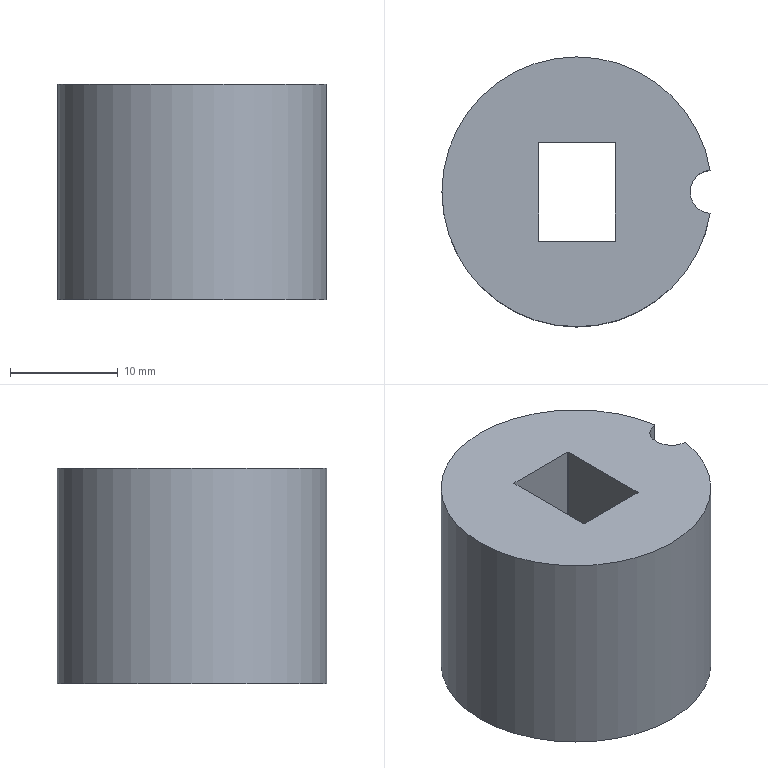Part | NX | features solid 2 | 1 solid | 14 faces | box 24.84 x 25 x 20 mm | volume 6576 mm3 | cylinder 7 | plane 7 | commonest cylinder face diameters 0.04 x4 4 x1 16.6 x1 25 x1
STEP:
#1=CARTESIAN_POINT('',(-372.16,213.243,2.596));
#2=VERTEX_POINT('',#1);
#3=CARTESIAN_POINT('',(-372.16,213.243,22.596));
#4=VERTEX_POINT('',#3);
#5=CARTESIAN_POINT('',(-372.16,213.243,12.596));
#6=DIRECTION('',(0.,0.,1.));
#7=VECTOR('',#6,1000.);
#8=LINE('',#5,#7);
#9=EDGE_CURVE('',#2,#4,#8,.T.);
#10=ORIENTED_EDGE('',*,*,#9,.T.);
#11=CARTESIAN_POINT('',(-372.16,217.23,22.596));
#12=VERTEX_POINT('',#11);
#13=CARTESIAN_POINT('',(-384.5,215.236,22.596));
#14=DIRECTION('',(0.,0.,-1.));
#15=DIRECTION('',(1.,0.,0.));
#16=AXIS2_PLACEMENT_3D('',#13,#14,#15);
#17=CIRCLE('',#16,12.5);
#18=EDGE_CURVE('',#4,#12,#17,.T.);
#19=ORIENTED_EDGE('',*,*,#18,.T.);
#20=CARTESIAN_POINT('',(-372.16,217.23,2.596));
#21=VERTEX_POINT('',#20);
#22=CARTESIAN_POINT('',(-372.16,217.23,12.596));
#23=DIRECTION('',(0.,0.,1.));
#24=VECTOR('',#23,1000.);
#25=LINE('',#22,#24);
#26=EDGE_CURVE('',#12,#21,#25,.F.);
#27=ORIENTED_EDGE('',*,*,#26,.T.);
#28=CARTESIAN_POINT('',(-384.5,215.236,2.596));
#29=DIRECTION('',(0.,0.,-1.));
#30=DIRECTION('',(1.,0.,0.));
#31=AXIS2_PLACEMENT_3D('',#28,#29,#30);
#32=CIRCLE('',#31,12.5);
#33=EDGE_CURVE('',#2,#21,#32,.T.);
#34=ORIENTED_EDGE('',*,*,#33,.F.);
#35=EDGE_LOOP('',(#10,#19,#27,#34));
#36=FACE_BOUND('',#35,.T.);
#37=CARTESIAN_POINT('',(-384.5,215.236,2.596));
#38=DIRECTION('',(0.,0.,1.));
#39=DIRECTION('',(1.,0.,0.));
#40=AXIS2_PLACEMENT_3D('',#37,#38,#39);
#41=CYLINDRICAL_SURFACE('',#40,12.5);
#42=ADVANCED_FACE('',(#36),#41,.T.);
#43=CARTESIAN_POINT('',(-376.2,215.236,2.596));
#44=VERTEX_POINT('',#43);
#45=CARTESIAN_POINT('',(-384.5,215.236,2.596));
#46=DIRECTION('',(0.,0.,-1.));
#47=DIRECTION('',(1.,0.,0.));
#48=AXIS2_PLACEMENT_3D('',#45,#46,#47);
#49=CIRCLE('',#48,8.3);
#50=EDGE_CURVE('',#44,#44,#49,.T.);
#51=ORIENTED_EDGE('',*,*,#50,.F.);
#52=EDGE_LOOP('',(#51));
#53=FACE_BOUND('',#52,.T.);
#54=ORIENTED_EDGE('',*,*,#33,.T.);
#55=CARTESIAN_POINT('',(-372.,215.236,2.596));
#56=DIRECTION('',(0.,0.,-1.));
#57=DIRECTION('',(1.,0.,0.));
#58=AXIS2_PLACEMENT_3D('',#55,#56,#57);
#59=CIRCLE('',#58,2.);
#60=EDGE_CURVE('',#2,#21,#59,.T.);
#61=ORIENTED_EDGE('',*,*,#60,.F.);
#62=EDGE_LOOP('',(#54,#61));
#63=FACE_BOUND('',#62,.T.);
#64=CARTESIAN_POINT('',(-384.5,215.236,2.596));
#65=DIRECTION('',(0.,0.,1.));
#66=DIRECTION('',(1.,0.,0.));
#67=AXIS2_PLACEMENT_3D('',#64,#65,#66);
#68=PLANE('',#67);
#69=ADVANCED_FACE('',(#53,#63),#68,.F.);
#70=CARTESIAN_POINT('',(-388.05,210.656,22.596));
#71=VERTEX_POINT('',#70);
#72=CARTESIAN_POINT('',(-388.05,219.816,22.596));
#73=VERTEX_POINT('',#72);
#74=CARTESIAN_POINT('',(-388.05,210.636,22.596));
#75=DIRECTION('',(0.,1.,0.));
#76=VECTOR('',#75,1000.);
#77=LINE('',#74,#76);
#78=EDGE_CURVE('',#71,#73,#77,.T.);
#79=ORIENTED_EDGE('',*,*,#78,.T.);
#80=CARTESIAN_POINT('',(-388.03,219.836,22.596));
#81=VERTEX_POINT('',#80);
#82=CARTESIAN_POINT('',(-388.03,219.816,22.596));
#83=DIRECTION('',(0.,0.,-1.));
#84=DIRECTION('',(1.,0.,0.));
#85=AXIS2_PLACEMENT_3D('',#82,#83,#84);
#86=CIRCLE('',#85,0.02);
#87=EDGE_CURVE('',#81,#73,#86,.F.);
#88=ORIENTED_EDGE('',*,*,#87,.F.);
#89=CARTESIAN_POINT('',(-380.97,219.836,22.596));
#90=VERTEX_POINT('',#89);
#91=CARTESIAN_POINT('',(-388.05,219.836,22.596));
#92=DIRECTION('',(1.,0.,0.));
#93=VECTOR('',#92,1000.);
#94=LINE('',#91,#93);
#95=EDGE_CURVE('',#81,#90,#94,.T.);
#96=ORIENTED_EDGE('',*,*,#95,.T.);
#97=CARTESIAN_POINT('',(-380.95,219.816,22.596));
#98=VERTEX_POINT('',#97);
#99=CARTESIAN_POINT('',(-380.97,219.816,22.596));
#100=DIRECTION('',(0.,0.,-1.));
#101=DIRECTION('',(1.,0.,0.));
#102=AXIS2_PLACEMENT_3D('',#99,#100,#101);
#103=CIRCLE('',#102,0.02);
#104=EDGE_CURVE('',#98,#90,#103,.F.);
#105=ORIENTED_EDGE('',*,*,#104,.F.);
#106=CARTESIAN_POINT('',(-380.95,210.656,22.596));
#107=VERTEX_POINT('',#106);
#108=CARTESIAN_POINT('',(-380.95,210.636,22.596));
#109=DIRECTION('',(0.,1.,0.));
#110=VECTOR('',#109,1000.);
#111=LINE('',#108,#110);
#112=EDGE_CURVE('',#107,#98,#111,.T.);
#113=ORIENTED_EDGE('',*,*,#112,.F.);
#114=CARTESIAN_POINT('',(-380.97,210.636,22.596));
#115=VERTEX_POINT('',#114);
#116=CARTESIAN_POINT('',(-380.97,210.656,22.596));
#117=DIRECTION('',(0.,0.,-1.));
#118=DIRECTION('',(1.,0.,0.));
#119=AXIS2_PLACEMENT_3D('',#116,#117,#118);
#120=CIRCLE('',#119,0.02);
#121=EDGE_CURVE('',#115,#107,#120,.F.);
#122=ORIENTED_EDGE('',*,*,#121,.F.);
#123=CARTESIAN_POINT('',(-388.03,210.636,22.596));
#124=VERTEX_POINT('',#123);
#125=CARTESIAN_POINT('',(-380.95,210.636,22.596));
#126=DIRECTION('',(-1.,0.,0.));
#127=VECTOR('',#126,1000.);
#128=LINE('',#125,#127);
#129=EDGE_CURVE('',#115,#124,#128,.T.);
#130=ORIENTED_EDGE('',*,*,#129,.T.);
#131=CARTESIAN_POINT('',(-388.03,210.656,22.596));
#132=DIRECTION('',(0.,0.,-1.));
#133=DIRECTION('',(1.,0.,0.));
#134=AXIS2_PLACEMENT_3D('',#131,#132,#133);
#135=CIRCLE('',#134,0.02);
#136=EDGE_CURVE('',#71,#124,#135,.F.);
#137=ORIENTED_EDGE('',*,*,#136,.F.);
#138=EDGE_LOOP('',(#79,#88,#96,#105,#113,#122,#130,#137));
#139=FACE_BOUND('',#138,.T.);
#140=CARTESIAN_POINT('',(-372.,215.236,22.596));
#141=DIRECTION('',(0.,0.,-1.));
#142=DIRECTION('',(1.,0.,0.));
#143=AXIS2_PLACEMENT_3D('',#140,#141,#142);
#144=CIRCLE('',#143,2.);
#145=EDGE_CURVE('',#4,#12,#144,.T.);
#146=ORIENTED_EDGE('',*,*,#145,.T.);
#147=ORIENTED_EDGE('',*,*,#18,.F.);
#148=EDGE_LOOP('',(#146,#147));
#149=FACE_BOUND('',#148,.T.);
#150=CARTESIAN_POINT('',(-384.5,215.236,22.596));
#151=DIRECTION('',(0.,0.,1.));
#152=DIRECTION('',(1.,0.,0.));
#153=AXIS2_PLACEMENT_3D('',#150,#151,#152);
#154=PLANE('',#153);
#155=ADVANCED_FACE('',(#139,#149),#154,.T.);
#156=ORIENTED_EDGE('',*,*,#50,.T.);
#157=EDGE_LOOP('',(#156));
#158=FACE_BOUND('',#157,.T.);
#159=CARTESIAN_POINT('',(-376.2,215.236,14.596));
#160=VERTEX_POINT('',#159);
#161=CARTESIAN_POINT('',(-384.5,215.236,14.596));
#162=DIRECTION('',(0.,0.,-1.));
#163=DIRECTION('',(1.,0.,0.));
#164=AXIS2_PLACEMENT_3D('',#161,#162,#163);
#165=CIRCLE('',#164,8.3);
#166=EDGE_CURVE('',#160,#160,#165,.T.);
#167=ORIENTED_EDGE('',*,*,#166,.F.);
#168=EDGE_LOOP('',(#167));
#169=FACE_BOUND('',#168,.T.);
#170=CARTESIAN_POINT('',(-384.5,215.236,2.596));
#171=DIRECTION('',(0.,0.,1.));
#172=DIRECTION('',(1.,0.,0.));
#173=AXIS2_PLACEMENT_3D('',#170,#171,#172);
#174=CYLINDRICAL_SURFACE('',#173,8.3);
#175=ADVANCED_FACE('',(#158,#169),#174,.F.);
#176=CARTESIAN_POINT('',(-380.95,210.656,14.596));
#177=VERTEX_POINT('',#176);
#178=CARTESIAN_POINT('',(-380.95,219.816,14.596));
#179=VERTEX_POINT('',#178);
#180=CARTESIAN_POINT('',(-380.95,215.236,14.596));
#181=DIRECTION('',(0.,1.,0.));
#182=VECTOR('',#181,1000.);
#183=LINE('',#180,#182);
#184=EDGE_CURVE('',#177,#179,#183,.T.);
#185=ORIENTED_EDGE('',*,*,#184,.T.);
#186=CARTESIAN_POINT('',(-380.97,219.836,14.596));
#187=VERTEX_POINT('',#186);
#188=CARTESIAN_POINT('',(-380.97,219.816,14.596));
#189=DIRECTION('',(0.,0.,-1.));
#190=DIRECTION('',(1.,0.,0.));
#191=AXIS2_PLACEMENT_3D('',#188,#189,#190);
#192=CIRCLE('',#191,0.02);
#193=EDGE_CURVE('',#187,#179,#192,.T.);
#194=ORIENTED_EDGE('',*,*,#193,.F.);
#195=CARTESIAN_POINT('',(-388.03,219.836,14.596));
#196=VERTEX_POINT('',#195);
#197=CARTESIAN_POINT('',(-384.5,219.836,14.596));
#198=DIRECTION('',(1.,0.,0.));
#199=VECTOR('',#198,1000.);
#200=LINE('',#197,#199);
#201=EDGE_CURVE('',#196,#187,#200,.T.);
#202=ORIENTED_EDGE('',*,*,#201,.F.);
#203=CARTESIAN_POINT('',(-388.05,219.816,14.596));
#204=VERTEX_POINT('',#203);
#205=CARTESIAN_POINT('',(-388.03,219.816,14.596));
#206=DIRECTION('',(0.,0.,-1.));
#207=DIRECTION('',(1.,0.,0.));
#208=AXIS2_PLACEMENT_3D('',#205,#206,#207);
#209=CIRCLE('',#208,0.02);
#210=EDGE_CURVE('',#204,#196,#209,.T.);
#211=ORIENTED_EDGE('',*,*,#210,.F.);
#212=CARTESIAN_POINT('',(-388.05,210.656,14.596));
#213=VERTEX_POINT('',#212);
#214=CARTESIAN_POINT('',(-388.05,215.236,14.596));
#215=DIRECTION('',(0.,1.,0.));
#216=VECTOR('',#215,1000.);
#217=LINE('',#214,#216);
#218=EDGE_CURVE('',#213,#204,#217,.T.);
#219=ORIENTED_EDGE('',*,*,#218,.F.);
#220=CARTESIAN_POINT('',(-388.03,210.636,14.596));
#221=VERTEX_POINT('',#220);
#222=CARTESIAN_POINT('',(-388.03,210.656,14.596));
#223=DIRECTION('',(0.,0.,-1.));
#224=DIRECTION('',(1.,0.,0.));
#225=AXIS2_PLACEMENT_3D('',#222,#223,#224);
#226=CIRCLE('',#225,0.02);
#227=EDGE_CURVE('',#221,#213,#226,.T.);
#228=ORIENTED_EDGE('',*,*,#227,.F.);
#229=CARTESIAN_POINT('',(-380.97,210.636,14.596));
#230=VERTEX_POINT('',#229);
#231=CARTESIAN_POINT('',(-384.5,210.636,14.596));
#232=DIRECTION('',(-1.,0.,0.));
#233=VECTOR('',#232,1000.);
#234=LINE('',#231,#233);
#235=EDGE_CURVE('',#230,#221,#234,.T.);
#236=ORIENTED_EDGE('',*,*,#235,.F.);
#237=CARTESIAN_POINT('',(-380.97,210.656,14.596));
#238=DIRECTION('',(0.,0.,-1.));
#239=DIRECTION('',(1.,0.,0.));
#240=AXIS2_PLACEMENT_3D('',#237,#238,#239);
#241=CIRCLE('',#240,0.02);
#242=EDGE_CURVE('',#177,#230,#241,.T.);
#243=ORIENTED_EDGE('',*,*,#242,.F.);
#244=EDGE_LOOP('',(#185,#194,#202,#211,#219,#228,#236,#243));
#245=FACE_BOUND('',#244,.T.);
#246=ORIENTED_EDGE('',*,*,#166,.T.);
#247=EDGE_LOOP('',(#246));
#248=FACE_BOUND('',#247,.T.);
#249=CARTESIAN_POINT('',(-384.5,215.236,14.596));
#250=DIRECTION('',(0.,0.,1.));
#251=DIRECTION('',(1.,0.,0.));
#252=AXIS2_PLACEMENT_3D('',#249,#250,#251);
#253=PLANE('',#252);
#254=ADVANCED_FACE('',(#245,#248),#253,.F.);
#255=ORIENTED_EDGE('',*,*,#9,.F.);
#256=ORIENTED_EDGE('',*,*,#60,.T.);
#257=ORIENTED_EDGE('',*,*,#26,.F.);
#258=ORIENTED_EDGE('',*,*,#145,.F.);
#259=EDGE_LOOP('',(#255,#256,#257,#258));
#260=FACE_BOUND('',#259,.T.);
#261=CARTESIAN_POINT('',(-372.,215.236,2.596));
#262=DIRECTION('',(0.,0.,1.));
#263=DIRECTION('',(1.,0.,0.));
#264=AXIS2_PLACEMENT_3D('',#261,#262,#263);
#265=CYLINDRICAL_SURFACE('',#264,2.);
#266=ADVANCED_FACE('',(#260),#265,.F.);
#267=ORIENTED_EDGE('',*,*,#78,.F.);
#268=CARTESIAN_POINT('',(-388.05,210.656,22.596));
#269=DIRECTION('',(0.,0.,1.));
#270=VECTOR('',#269,1000.);
#271=LINE('',#268,#270);
#272=EDGE_CURVE('',#213,#71,#271,.T.);
#273=ORIENTED_EDGE('',*,*,#272,.F.);
#274=ORIENTED_EDGE('',*,*,#218,.T.);
#275=CARTESIAN_POINT('',(-388.05,219.816,14.596));
#276=DIRECTION('',(0.,0.,1.));
#277=VECTOR('',#276,1000.);
#278=LINE('',#275,#277);
#279=EDGE_CURVE('',#73,#204,#278,.F.);
#280=ORIENTED_EDGE('',*,*,#279,.F.);
#281=EDGE_LOOP('',(#267,#273,#274,#280));
#282=FACE_BOUND('',#281,.T.);
#283=CARTESIAN_POINT('',(-388.05,210.636,2.596));
#284=DIRECTION('',(-1.,0.,0.));
#285=DIRECTION('',(0.,0.,1.));
#286=AXIS2_PLACEMENT_3D('',#283,#284,#285);
#287=PLANE('',#286);
#288=ADVANCED_FACE('',(#282),#287,.F.);
#289=ORIENTED_EDGE('',*,*,#95,.F.);
#290=CARTESIAN_POINT('',(-388.03,219.836,22.596));
#291=DIRECTION('',(0.,0.,1.));
#292=VECTOR('',#291,1000.);
#293=LINE('',#290,#292);
#294=EDGE_CURVE('',#196,#81,#293,.T.);
#295=ORIENTED_EDGE('',*,*,#294,.F.);
#296=ORIENTED_EDGE('',*,*,#201,.T.);
#297=CARTESIAN_POINT('',(-380.97,219.836,2.596));
#298=DIRECTION('',(0.,0.,1.));
#299=VECTOR('',#298,1000.);
#300=LINE('',#297,#299);
#301=EDGE_CURVE('',#90,#187,#300,.F.);
#302=ORIENTED_EDGE('',*,*,#301,.F.);
#303=EDGE_LOOP('',(#289,#295,#296,#302));
#304=FACE_BOUND('',#303,.T.);
#305=CARTESIAN_POINT('',(-388.05,219.836,2.596));
#306=DIRECTION('',(0.,1.,0.));
#307=DIRECTION('',(0.,0.,-1.));
#308=AXIS2_PLACEMENT_3D('',#305,#306,#307);
#309=PLANE('',#308);
#310=ADVANCED_FACE('',(#304),#309,.F.);
#311=ORIENTED_EDGE('',*,*,#112,.T.);
#312=CARTESIAN_POINT('',(-380.95,219.816,2.596));
#313=DIRECTION('',(0.,0.,1.));
#314=VECTOR('',#313,1000.);
#315=LINE('',#312,#314);
#316=EDGE_CURVE('',#179,#98,#315,.T.);
#317=ORIENTED_EDGE('',*,*,#316,.F.);
#318=ORIENTED_EDGE('',*,*,#184,.F.);
#319=CARTESIAN_POINT('',(-380.95,210.656,2.596));
#320=DIRECTION('',(0.,0.,1.));
#321=VECTOR('',#320,1000.);
#322=LINE('',#319,#321);
#323=EDGE_CURVE('',#107,#177,#322,.F.);
#324=ORIENTED_EDGE('',*,*,#323,.F.);
#325=EDGE_LOOP('',(#311,#317,#318,#324));
#326=FACE_BOUND('',#325,.T.);
#327=CARTESIAN_POINT('',(-380.95,210.636,2.596));
#328=DIRECTION('',(-1.,0.,0.));
#329=DIRECTION('',(0.,0.,1.));
#330=AXIS2_PLACEMENT_3D('',#327,#328,#329);
#331=PLANE('',#330);
#332=ADVANCED_FACE('',(#326),#331,.T.);
#333=ORIENTED_EDGE('',*,*,#235,.T.);
#334=CARTESIAN_POINT('',(-388.03,210.636,14.596));
#335=DIRECTION('',(0.,0.,1.));
#336=VECTOR('',#335,1000.);
#337=LINE('',#334,#336);
#338=EDGE_CURVE('',#124,#221,#337,.F.);
#339=ORIENTED_EDGE('',*,*,#338,.F.);
#340=ORIENTED_EDGE('',*,*,#129,.F.);
#341=CARTESIAN_POINT('',(-380.97,210.636,2.596));
#342=DIRECTION('',(0.,0.,1.));
#343=VECTOR('',#342,1000.);
#344=LINE('',#341,#343);
#345=EDGE_CURVE('',#230,#115,#344,.T.);
#346=ORIENTED_EDGE('',*,*,#345,.F.);
#347=EDGE_LOOP('',(#333,#339,#340,#346));
#348=FACE_BOUND('',#347,.T.);
#349=CARTESIAN_POINT('',(-380.95,210.636,2.596));
#350=DIRECTION('',(0.,-1.,0.));
#351=DIRECTION('',(0.,0.,1.));
#352=AXIS2_PLACEMENT_3D('',#349,#350,#351);
#353=PLANE('',#352);
#354=ADVANCED_FACE('',(#348),#353,.F.);
#355=ORIENTED_EDGE('',*,*,#242,.T.);
#356=ORIENTED_EDGE('',*,*,#345,.T.);
#357=ORIENTED_EDGE('',*,*,#121,.T.);
#358=ORIENTED_EDGE('',*,*,#323,.T.);
#359=EDGE_LOOP('',(#355,#356,#357,#358));
#360=FACE_BOUND('',#359,.T.);
#361=CARTESIAN_POINT('',(-380.97,210.656,2.596));
#362=DIRECTION('',(0.,0.,1.));
#363=DIRECTION('',(1.,0.,0.));
#364=AXIS2_PLACEMENT_3D('',#361,#362,#363);
#365=CYLINDRICAL_SURFACE('',#364,0.02);
#366=ADVANCED_FACE('',(#360),#365,.F.);
#367=ORIENTED_EDGE('',*,*,#193,.T.);
#368=ORIENTED_EDGE('',*,*,#316,.T.);
#369=ORIENTED_EDGE('',*,*,#104,.T.);
#370=ORIENTED_EDGE('',*,*,#301,.T.);
#371=EDGE_LOOP('',(#367,#368,#369,#370));
#372=FACE_BOUND('',#371,.T.);
#373=CARTESIAN_POINT('',(-380.97,219.816,2.596));
#374=DIRECTION('',(0.,0.,1.));
#375=DIRECTION('',(1.,0.,0.));
#376=AXIS2_PLACEMENT_3D('',#373,#374,#375);
#377=CYLINDRICAL_SURFACE('',#376,0.02);
#378=ADVANCED_FACE('',(#372),#377,.F.);
#379=ORIENTED_EDGE('',*,*,#210,.T.);
#380=ORIENTED_EDGE('',*,*,#294,.T.);
#381=ORIENTED_EDGE('',*,*,#87,.T.);
#382=ORIENTED_EDGE('',*,*,#279,.T.);
#383=EDGE_LOOP('',(#379,#380,#381,#382));
#384=FACE_BOUND('',#383,.T.);
#385=CARTESIAN_POINT('',(-388.03,219.816,2.596));
#386=DIRECTION('',(0.,0.,-1.));
#387=DIRECTION('',(-1.,0.,0.));
#388=AXIS2_PLACEMENT_3D('',#385,#386,#387);
#389=CYLINDRICAL_SURFACE('',#388,0.02);
#390=ADVANCED_FACE('',(#384),#389,.F.);
#391=ORIENTED_EDGE('',*,*,#227,.T.);
#392=ORIENTED_EDGE('',*,*,#272,.T.);
#393=ORIENTED_EDGE('',*,*,#136,.T.);
#394=ORIENTED_EDGE('',*,*,#338,.T.);
#395=EDGE_LOOP('',(#391,#392,#393,#394));
#396=FACE_BOUND('',#395,.T.);
#397=CARTESIAN_POINT('',(-388.03,210.656,2.596));
#398=DIRECTION('',(0.,0.,-1.));
#399=DIRECTION('',(-1.,0.,0.));
#400=AXIS2_PLACEMENT_3D('',#397,#398,#399);
#401=CYLINDRICAL_SURFACE('',#400,0.02);
#402=ADVANCED_FACE('',(#396),#401,.F.);
#403=CLOSED_SHELL('',(#42,#69,#155,#175,#254,#266,#288,#310,#332,#354,#366,#378,#390,#402));
#404=MANIFOLD_SOLID_BREP('',#403);
#405=(LENGTH_UNIT()NAMED_UNIT(*)SI_UNIT(.MILLI.,.METRE.));
#406=UNCERTAINTY_MEASURE_WITH_UNIT(LENGTH_MEASURE(0.00001),#405,'','');
#407=(NAMED_UNIT(*)PLANE_ANGLE_UNIT()SI_UNIT($,.RADIAN.));
#408=(NAMED_UNIT(*)SI_UNIT($,.STERADIAN.)SOLID_ANGLE_UNIT());
#409=(GEOMETRIC_REPRESENTATION_CONTEXT(3)GLOBAL_UNCERTAINTY_ASSIGNED_CONTEXT((#406))GLOBAL_UNIT_ASSIGNED_CONTEXT((#405,#407,#408))REPRESENTATION_CONTEXT('',''));
#410=ADVANCED_BREP_SHAPE_REPRESENTATION('',(#404),#409);